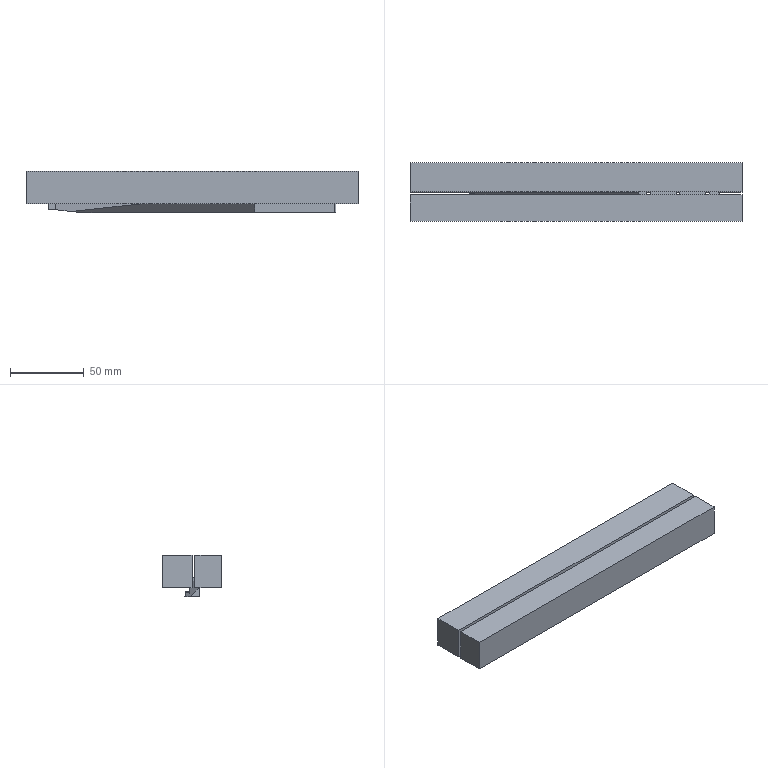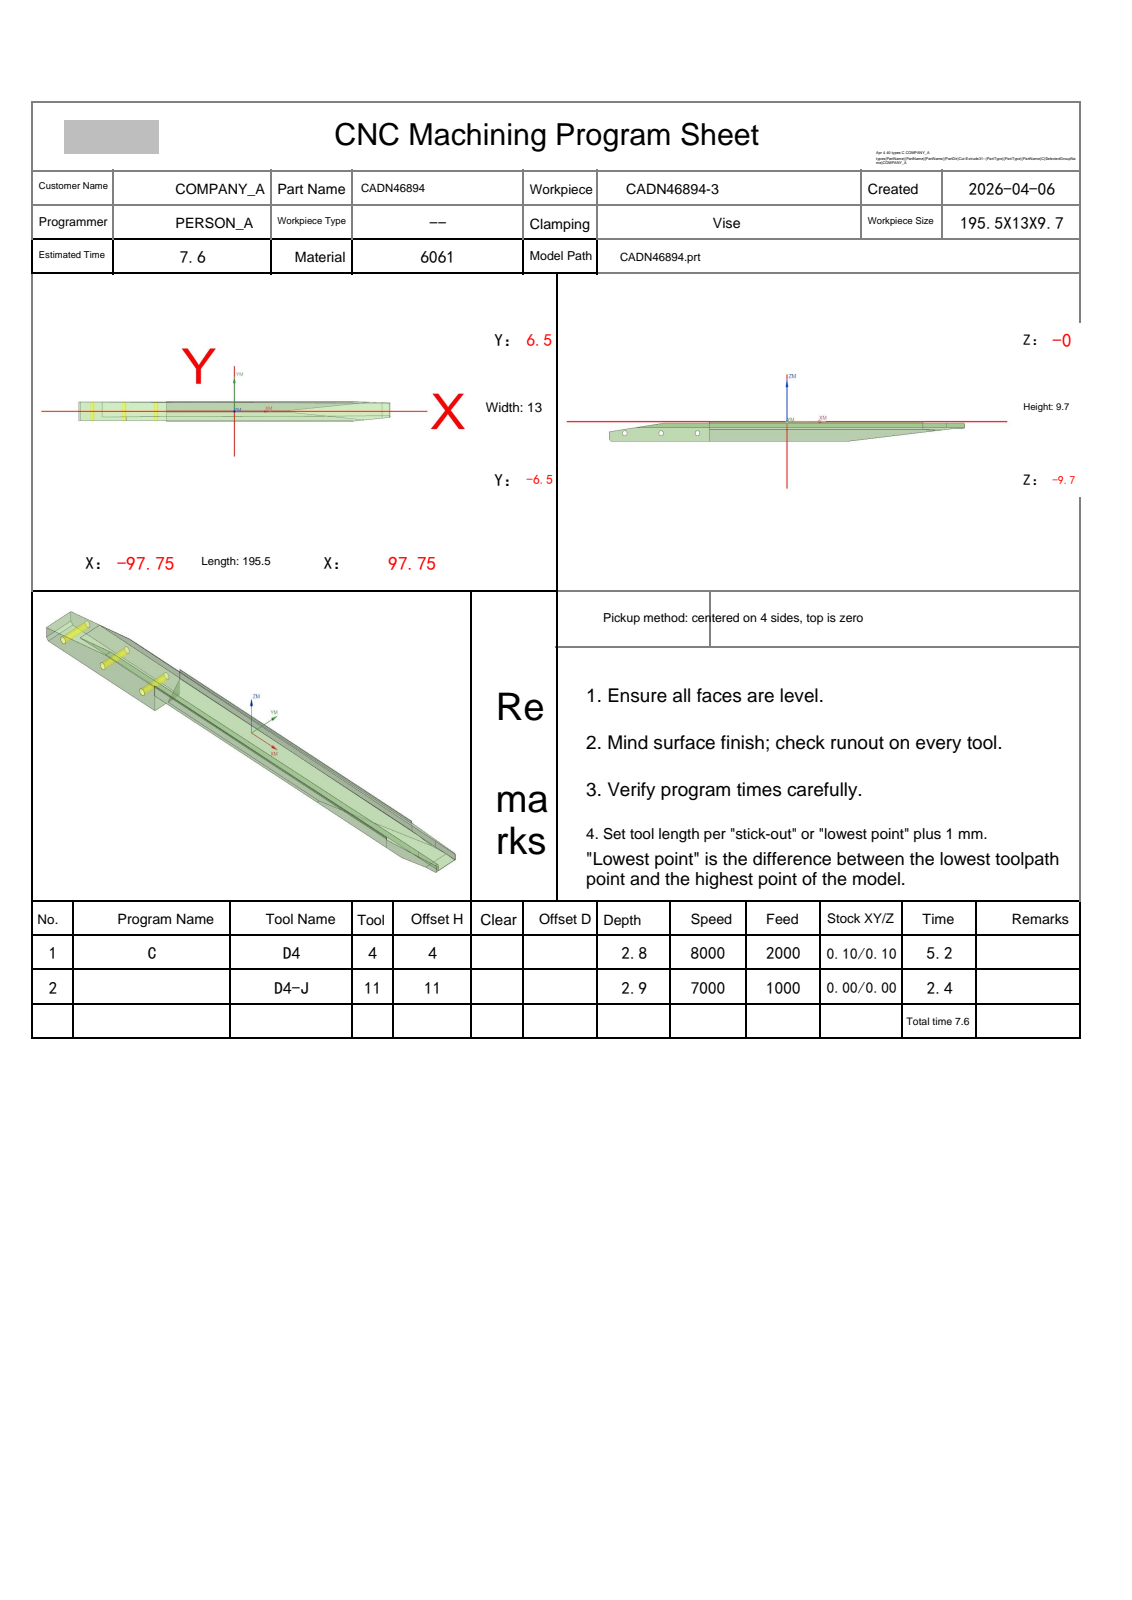NC program | NX | posted by the shop | part box 225.5 x 39.7 x 28 mm
Lines 19948 to 20119 of 20119:
N4 T02 M06
(D6 chamfer tool  D=6. R=0. H=02 ce=0.00 di=0.00)
G00 G90 G54 X-194.273 Y-6.464 M03 S6500
G43 H02 Z44.
M08
Z-5.887
G01 Z-7.2 F1500.
G03 X-194.473 Y-6.75 I1.532 J-1.286
G01 X-194.503 Y-6.796
X-194.5 Y-6.85
Y-7.968
G02 X-195.219 Y-9.504 I-2. J0.0
X-192.5 Y-8.7 I2.719 J-4.196
G01 X-65.732
G02 X-64. Y-9.7 I0.0 J-2.
X-62.386 Y-8.519 I1.83 J-.807
G01 X-37.834 Y-5.856
X-37.78 Y-5.853
X-37.738 Y-5.818
G03 X-37.476 Y-5.589 I-1.181 J1.614
G01 Z-5.863
G00 Z4.
X-19.805 Y-3.672
Z-5.887
G01 Z-7.2
G03 X-19.499 Y-3.84 I1.113 J1.662
G01 X-19.451 Y-3.865
X-19.397 Y-3.856
X-5.108 Y-2.306
X-5.054 Y-2.301
X-5. Y-2.3
X-3.
X-2.439 Y-2.332
X-1.885 Y-2.426
X-1.346 Y-2.582
X-.827 Y-2.797
X-.922 Y-2.612
X-.98 Y-2.412
X-1. Y-2.205
Y-1.795
X-.98 Y-1.588
X-.922 Y-1.388
X-.827 Y-1.203
X-1.346 Y-1.418
X-1.885 Y-1.574
X-2.439 Y-1.668
X-3. Y-1.7
X-19.2
X-19.459 Y-1.666
X-19.7 Y-1.566
X-19.907 Y-1.407
X-20.314 Y-1.
X-143.186
X-143.593 Y-1.407
X-143.8 Y-1.566
X-144.041 Y-1.666
X-144.3 Y-1.7
X-163.768
G02 X-165.5 Y-.7 I0.0 J2.
X-167.073 Y-1.936 I-1.856 J.744
G01 X-194.312 Y-5.84
X-194.366 Y-5.845
X-194.407 Y-5.881
G03 X-194.661 Y-6.119 I1.236 J-1.573
G01 Z-5.714
G00 Z44.
G91 G28 Z0.0
M05
M09
G91 G28 Z0.0
M01
N5 T17 M06
(D2-J  D=2. R=0. H=17 ce=0.00 di=0.00)
G00 G90 G54 X-192.907 Y-8.115 M03 S8000
G43 H17 Z4.
M08
Z-7.133
G01 Z-8.133 F800.
G41 D17
X-192.9 Y-8.315
G03 X-192.5 Y-8.7 I.4 J.015
G01 X-65.732
G02 X-65.076 Y-8.811 I0.0 J-2.
G01 X-5.054 Y-2.3
X-3.
G02 X-.827 Y-2.797 I0.0 J-5.
X-1. Y-2.205 I.927 J.592
G01 Y-1.795
G02 X-.827 Y-1.203 I1.1 J0.0
X-3. Y-1.7 I-2.173 J4.503
G01 X-19.614
X-20.314 Y-1.
X-143.186
X-143.886 Y-1.7
X-163.768
G02 X-165.5 Y-.7 I0.0 J2.
X-167.073 Y-1.936 I-1.856 J.744
G01 X-194.5 Y-5.867
Y-7.968
G02 X-195.219 Y-9.504 I-2. J0.0
X-192.5 Y-8.7 I2.719 J-4.196
G01 X-192.1
G03 X-191.7 Y-8.3 I0.0 J.4
G01 G40 Y-8.1
Z-7.133
G00 X-192.907 Y-8.115
Z-9.267
G01 Z-10.267
G41 D17
X-192.9 Y-8.315
G03 X-192.5 Y-8.7 I.4 J.015
G01 X-65.732
G02 X-65.076 Y-8.811 I0.0 J-2.
G01 X-5.054 Y-2.3
X-3.
G02 X-.827 Y-2.797 I0.0 J-5.
X-1. Y-2.205 I.927 J.592
G01 Y-1.795
G02 X-.827 Y-1.203 I1.1 J0.0
X-3. Y-1.7 I-2.173 J4.503
G01 X-19.614
X-20.314 Y-1.
X-143.186
X-143.886 Y-1.7
X-163.768
G02 X-165.5 Y-.7 I0.0 J2.
X-167.073 Y-1.936 I-1.856 J.744
G01 X-194.5 Y-5.867
Y-7.968
G02 X-195.219 Y-9.504 I-2. J0.0
X-192.5 Y-8.7 I2.719 J-4.196
G01 X-192.1
G03 X-191.7 Y-8.3 I0.0 J.4
G01 G40 Y-8.1
Z-9.267
G00 X-192.907 Y-8.115
Z-11.4
G01 Z-12.4
G41 D17
X-192.9 Y-8.315
G03 X-192.5 Y-8.7 I.4 J.015
G01 X-65.732
G02 X-65.076 Y-8.811 I0.0 J-2.
G01 X-5.054 Y-2.3
X-3.
G02 X-.827 Y-2.797 I0.0 J-5.
X-1. Y-2.205 I.927 J.592
G01 Y-1.795
G02 X-.827 Y-1.203 I1.1 J0.0
X-3. Y-1.7 I-2.173 J4.503
G01 X-19.614
X-20.314 Y-1.
X-143.186
X-143.886 Y-1.7
X-163.768
G02 X-165.5 Y-.7 I0.0 J2.
X-167.073 Y-1.936 I-1.856 J.744
G01 X-194.5 Y-5.867
Y-7.968
G02 X-195.219 Y-9.504 I-2. J0.0
X-192.5 Y-8.7 I2.719 J-4.196
G01 X-192.1
G03 X-191.7 Y-8.3 I0.0 J.4
G01 G40 Y-8.1
Z-11.4
G00 Z4.
M05
M09
G91 G28 Z0.0
G91 G28 Y0.0
M30
%